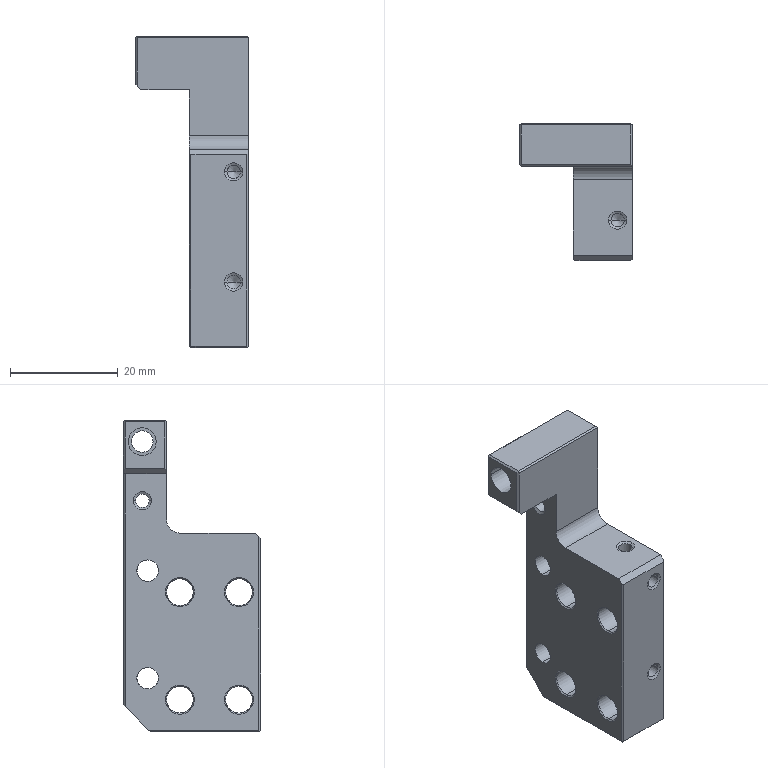Part | NX | 1 solid | 88 faces | box 21 x 25.5 x 58 mm | volume 11180 mm3 | cylinder 35 | plane 27 | cone 26 | commonest cylinder face diameters 2.5 x18 5 x9 4 x6 5.2 x2